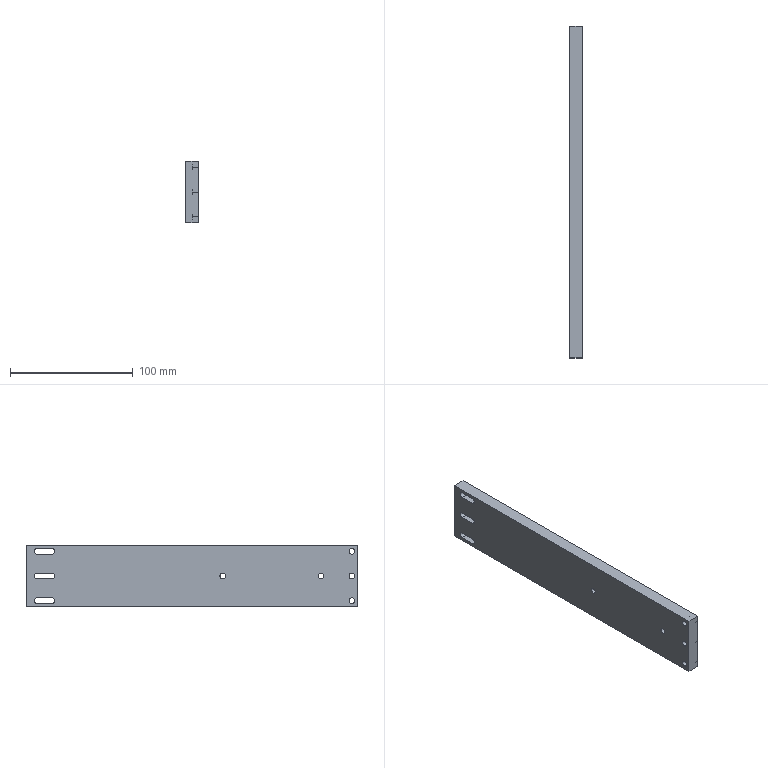Part | STEP file | 04-11 Guide cylinder raised bracket plate | 1 solid | 43 faces | box 10 x 270 x 50 mm | volume 130915 mm3 | cylinder 26 | plane 17 | commonest cylinder face diameters 4.5 x16 9 x10